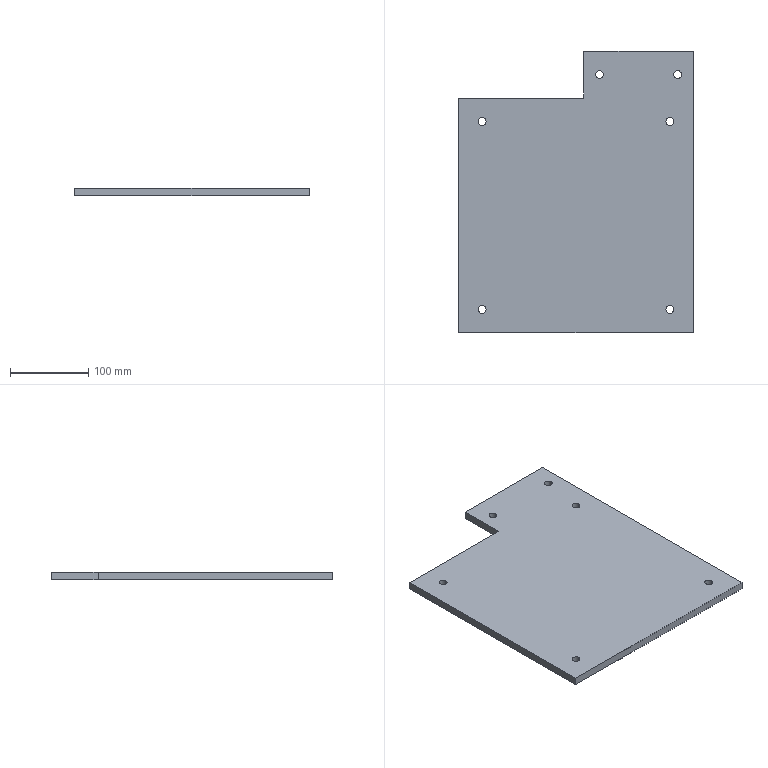Part | SolidWorks | features ICE 2, Extrusion 1 | 1 solid | 20 faces | box 300 x 360 x 10 mm | volume 979288 mm3 | cylinder 12 | plane 8 | commonest cylinder face diameters 10 x12
STEP:
#1=CARTESIAN_POINT('',(275.,330.,0.));
#2=VERTEX_POINT('',#1);
#3=CARTESIAN_POINT('',(285.,330.,0.));
#4=VERTEX_POINT('',#3);
#5=CARTESIAN_POINT('',(280.,330.,0.));
#6=DIRECTION('',(0.,0.,1.));
#7=DIRECTION('',(1.,0.,0.));
#8=AXIS2_PLACEMENT_3D('',#5,#6,#7);
#9=CIRCLE('',#8,5.);
#10=EDGE_CURVE('',#2,#4,#9,.T.);
#11=ORIENTED_EDGE('',*,*,#10,.F.);
#12=CARTESIAN_POINT('',(275.,330.,10.));
#13=VERTEX_POINT('',#12);
#14=CARTESIAN_POINT('',(275.,330.,-30.));
#15=DIRECTION('',(0.,0.,1.));
#16=VECTOR('',#15,1000.);
#17=LINE('',#14,#16);
#18=EDGE_CURVE('',#2,#13,#17,.T.);
#19=ORIENTED_EDGE('',*,*,#18,.T.);
#20=CARTESIAN_POINT('',(285.,330.,10.));
#21=VERTEX_POINT('',#20);
#22=CARTESIAN_POINT('',(280.,330.,10.));
#23=DIRECTION('',(0.,0.,1.));
#24=DIRECTION('',(1.,0.,0.));
#25=AXIS2_PLACEMENT_3D('',#22,#23,#24);
#26=CIRCLE('',#25,5.);
#27=EDGE_CURVE('',#13,#21,#26,.T.);
#28=ORIENTED_EDGE('',*,*,#27,.T.);
#29=CARTESIAN_POINT('',(285.,330.,-30.));
#30=DIRECTION('',(0.,0.,1.));
#31=VECTOR('',#30,1000.);
#32=LINE('',#29,#31);
#33=EDGE_CURVE('',#4,#21,#32,.T.);
#34=ORIENTED_EDGE('',*,*,#33,.F.);
#35=EDGE_LOOP('',(#11,#19,#28,#34));
#36=FACE_OUTER_BOUND('',#35,.T.);
#37=CARTESIAN_POINT('',(280.,330.,-30.));
#38=DIRECTION('',(0.,0.,1.));
#39=DIRECTION('',(1.,0.,0.));
#40=AXIS2_PLACEMENT_3D('',#37,#38,#39);
#41=CYLINDRICAL_SURFACE('',#40,5.);
#42=ADVANCED_FACE('',(#36),#41,.F.);
#43=CARTESIAN_POINT('',(185.,330.,0.));
#44=VERTEX_POINT('',#43);
#45=CARTESIAN_POINT('',(175.,330.,0.));
#46=VERTEX_POINT('',#45);
#47=CARTESIAN_POINT('',(180.,330.,0.));
#48=DIRECTION('',(0.,0.,-1.));
#49=DIRECTION('',(1.,0.,0.));
#50=AXIS2_PLACEMENT_3D('',#47,#48,#49);
#51=CIRCLE('',#50,5.);
#52=EDGE_CURVE('',#44,#46,#51,.T.);
#53=ORIENTED_EDGE('',*,*,#52,.T.);
#54=CARTESIAN_POINT('',(175.,330.,10.));
#55=VERTEX_POINT('',#54);
#56=CARTESIAN_POINT('',(175.,330.,-30.));
#57=DIRECTION('',(0.,0.,1.));
#58=VECTOR('',#57,1000.);
#59=LINE('',#56,#58);
#60=EDGE_CURVE('',#46,#55,#59,.T.);
#61=ORIENTED_EDGE('',*,*,#60,.T.);
#62=CARTESIAN_POINT('',(185.,330.,10.));
#63=VERTEX_POINT('',#62);
#64=CARTESIAN_POINT('',(180.,330.,10.));
#65=DIRECTION('',(0.,0.,-1.));
#66=DIRECTION('',(1.,0.,0.));
#67=AXIS2_PLACEMENT_3D('',#64,#65,#66);
#68=CIRCLE('',#67,5.);
#69=EDGE_CURVE('',#63,#55,#68,.T.);
#70=ORIENTED_EDGE('',*,*,#69,.F.);
#71=CARTESIAN_POINT('',(185.,330.,-30.));
#72=DIRECTION('',(0.,0.,1.));
#73=VECTOR('',#72,1000.);
#74=LINE('',#71,#73);
#75=EDGE_CURVE('',#44,#63,#74,.T.);
#76=ORIENTED_EDGE('',*,*,#75,.F.);
#77=EDGE_LOOP('',(#53,#61,#70,#76));
#78=FACE_OUTER_BOUND('',#77,.T.);
#79=CARTESIAN_POINT('',(180.,330.,-30.));
#80=DIRECTION('',(0.,0.,1.));
#81=DIRECTION('',(1.,0.,0.));
#82=AXIS2_PLACEMENT_3D('',#79,#80,#81);
#83=CYLINDRICAL_SURFACE('',#82,5.);
#84=ADVANCED_FACE('',(#78),#83,.F.);
#85=CARTESIAN_POINT('',(35.,270.,10.));
#86=VERTEX_POINT('',#85);
#87=CARTESIAN_POINT('',(25.,270.,10.));
#88=VERTEX_POINT('',#87);
#89=CARTESIAN_POINT('',(30.,270.,10.));
#90=DIRECTION('',(0.,0.,-1.));
#91=DIRECTION('',(1.,0.,0.));
#92=AXIS2_PLACEMENT_3D('',#89,#90,#91);
#93=CIRCLE('',#92,5.);
#94=EDGE_CURVE('',#86,#88,#93,.T.);
#95=ORIENTED_EDGE('',*,*,#94,.F.);
#96=CARTESIAN_POINT('',(35.,270.,0.));
#97=VERTEX_POINT('',#96);
#98=CARTESIAN_POINT('',(35.,270.,10.));
#99=DIRECTION('',(0.,0.,-1.));
#100=VECTOR('',#99,1000.);
#101=LINE('',#98,#100);
#102=EDGE_CURVE('',#86,#97,#101,.T.);
#103=ORIENTED_EDGE('',*,*,#102,.T.);
#104=CARTESIAN_POINT('',(25.,270.,0.));
#105=VERTEX_POINT('',#104);
#106=CARTESIAN_POINT('',(30.,270.,0.));
#107=DIRECTION('',(0.,0.,-1.));
#108=DIRECTION('',(1.,0.,0.));
#109=AXIS2_PLACEMENT_3D('',#106,#107,#108);
#110=CIRCLE('',#109,5.);
#111=EDGE_CURVE('',#97,#105,#110,.T.);
#112=ORIENTED_EDGE('',*,*,#111,.T.);
#113=CARTESIAN_POINT('',(25.,270.,10.));
#114=DIRECTION('',(0.,0.,-1.));
#115=VECTOR('',#114,1000.);
#116=LINE('',#113,#115);
#117=EDGE_CURVE('',#88,#105,#116,.T.);
#118=ORIENTED_EDGE('',*,*,#117,.F.);
#119=EDGE_LOOP('',(#95,#103,#112,#118));
#120=FACE_OUTER_BOUND('',#119,.T.);
#121=CARTESIAN_POINT('',(30.,270.,10.));
#122=DIRECTION('',(0.,0.,-1.));
#123=DIRECTION('',(-1.,0.,0.));
#124=AXIS2_PLACEMENT_3D('',#121,#122,#123);
#125=CYLINDRICAL_SURFACE('',#124,5.);
#126=ADVANCED_FACE('',(#120),#125,.F.);
#127=CARTESIAN_POINT('',(275.,30.,10.));
#128=VERTEX_POINT('',#127);
#129=CARTESIAN_POINT('',(265.,30.,10.));
#130=VERTEX_POINT('',#129);
#131=CARTESIAN_POINT('',(270.,30.,10.));
#132=DIRECTION('',(0.,0.,-1.));
#133=DIRECTION('',(1.,0.,0.));
#134=AXIS2_PLACEMENT_3D('',#131,#132,#133);
#135=CIRCLE('',#134,5.);
#136=EDGE_CURVE('',#128,#130,#135,.T.);
#137=ORIENTED_EDGE('',*,*,#136,.F.);
#138=CARTESIAN_POINT('',(275.,30.,0.));
#139=VERTEX_POINT('',#138);
#140=CARTESIAN_POINT('',(275.,30.,10.));
#141=DIRECTION('',(0.,0.,-1.));
#142=VECTOR('',#141,1000.);
#143=LINE('',#140,#142);
#144=EDGE_CURVE('',#128,#139,#143,.T.);
#145=ORIENTED_EDGE('',*,*,#144,.T.);
#146=CARTESIAN_POINT('',(265.,30.,0.));
#147=VERTEX_POINT('',#146);
#148=CARTESIAN_POINT('',(270.,30.,0.));
#149=DIRECTION('',(0.,0.,-1.));
#150=DIRECTION('',(1.,0.,0.));
#151=AXIS2_PLACEMENT_3D('',#148,#149,#150);
#152=CIRCLE('',#151,5.);
#153=EDGE_CURVE('',#139,#147,#152,.T.);
#154=ORIENTED_EDGE('',*,*,#153,.T.);
#155=CARTESIAN_POINT('',(265.,30.,10.));
#156=DIRECTION('',(0.,0.,-1.));
#157=VECTOR('',#156,1000.);
#158=LINE('',#155,#157);
#159=EDGE_CURVE('',#130,#147,#158,.T.);
#160=ORIENTED_EDGE('',*,*,#159,.F.);
#161=EDGE_LOOP('',(#137,#145,#154,#160));
#162=FACE_OUTER_BOUND('',#161,.T.);
#163=CARTESIAN_POINT('',(270.,30.,10.));
#164=DIRECTION('',(0.,0.,-1.));
#165=DIRECTION('',(-1.,0.,0.));
#166=AXIS2_PLACEMENT_3D('',#163,#164,#165);
#167=CYLINDRICAL_SURFACE('',#166,5.);
#168=ADVANCED_FACE('',(#162),#167,.F.);
#169=CARTESIAN_POINT('',(25.,30.,10.));
#170=VERTEX_POINT('',#169);
#171=CARTESIAN_POINT('',(35.,30.,10.));
#172=VERTEX_POINT('',#171);
#173=CARTESIAN_POINT('',(30.,30.,10.));
#174=DIRECTION('',(0.,0.,1.));
#175=DIRECTION('',(1.,0.,0.));
#176=AXIS2_PLACEMENT_3D('',#173,#174,#175);
#177=CIRCLE('',#176,5.);
#178=EDGE_CURVE('',#170,#172,#177,.T.);
#179=ORIENTED_EDGE('',*,*,#178,.T.);
#180=CARTESIAN_POINT('',(35.,30.,0.));
#181=VERTEX_POINT('',#180);
#182=CARTESIAN_POINT('',(35.,30.,10.));
#183=DIRECTION('',(0.,0.,-1.));
#184=VECTOR('',#183,1000.);
#185=LINE('',#182,#184);
#186=EDGE_CURVE('',#172,#181,#185,.T.);
#187=ORIENTED_EDGE('',*,*,#186,.T.);
#188=CARTESIAN_POINT('',(25.,30.,0.));
#189=VERTEX_POINT('',#188);
#190=CARTESIAN_POINT('',(30.,30.,0.));
#191=DIRECTION('',(0.,0.,1.));
#192=DIRECTION('',(1.,0.,0.));
#193=AXIS2_PLACEMENT_3D('',#190,#191,#192);
#194=CIRCLE('',#193,5.);
#195=EDGE_CURVE('',#189,#181,#194,.T.);
#196=ORIENTED_EDGE('',*,*,#195,.F.);
#197=CARTESIAN_POINT('',(25.,30.,10.));
#198=DIRECTION('',(0.,0.,-1.));
#199=VECTOR('',#198,1000.);
#200=LINE('',#197,#199);
#201=EDGE_CURVE('',#170,#189,#200,.T.);
#202=ORIENTED_EDGE('',*,*,#201,.F.);
#203=EDGE_LOOP('',(#179,#187,#196,#202));
#204=FACE_OUTER_BOUND('',#203,.T.);
#205=CARTESIAN_POINT('',(30.,30.,10.));
#206=DIRECTION('',(0.,0.,-1.));
#207=DIRECTION('',(-1.,0.,0.));
#208=AXIS2_PLACEMENT_3D('',#205,#206,#207);
#209=CYLINDRICAL_SURFACE('',#208,5.);
#210=ADVANCED_FACE('',(#204),#209,.F.);
#211=CARTESIAN_POINT('',(265.,270.,10.));
#212=VERTEX_POINT('',#211);
#213=CARTESIAN_POINT('',(275.,270.,10.));
#214=VERTEX_POINT('',#213);
#215=CARTESIAN_POINT('',(270.,270.,10.));
#216=DIRECTION('',(0.,0.,1.));
#217=DIRECTION('',(1.,0.,0.));
#218=AXIS2_PLACEMENT_3D('',#215,#216,#217);
#219=CIRCLE('',#218,5.);
#220=EDGE_CURVE('',#212,#214,#219,.T.);
#221=ORIENTED_EDGE('',*,*,#220,.T.);
#222=CARTESIAN_POINT('',(275.,270.,0.));
#223=VERTEX_POINT('',#222);
#224=CARTESIAN_POINT('',(275.,270.,10.));
#225=DIRECTION('',(0.,0.,-1.));
#226=VECTOR('',#225,1000.);
#227=LINE('',#224,#226);
#228=EDGE_CURVE('',#214,#223,#227,.T.);
#229=ORIENTED_EDGE('',*,*,#228,.T.);
#230=CARTESIAN_POINT('',(265.,270.,0.));
#231=VERTEX_POINT('',#230);
#232=CARTESIAN_POINT('',(270.,270.,0.));
#233=DIRECTION('',(0.,0.,1.));
#234=DIRECTION('',(1.,0.,0.));
#235=AXIS2_PLACEMENT_3D('',#232,#233,#234);
#236=CIRCLE('',#235,5.);
#237=EDGE_CURVE('',#231,#223,#236,.T.);
#238=ORIENTED_EDGE('',*,*,#237,.F.);
#239=CARTESIAN_POINT('',(265.,270.,10.));
#240=DIRECTION('',(0.,0.,-1.));
#241=VECTOR('',#240,1000.);
#242=LINE('',#239,#241);
#243=EDGE_CURVE('',#212,#231,#242,.T.);
#244=ORIENTED_EDGE('',*,*,#243,.F.);
#245=EDGE_LOOP('',(#221,#229,#238,#244));
#246=FACE_OUTER_BOUND('',#245,.T.);
#247=CARTESIAN_POINT('',(270.,270.,10.));
#248=DIRECTION('',(0.,0.,-1.));
#249=DIRECTION('',(-1.,0.,0.));
#250=AXIS2_PLACEMENT_3D('',#247,#248,#249);
#251=CYLINDRICAL_SURFACE('',#250,5.);
#252=ADVANCED_FACE('',(#246),#251,.F.);
#253=CARTESIAN_POINT('',(280.,330.,10.));
#254=DIRECTION('',(0.,0.,1.));
#255=DIRECTION('',(1.,0.,0.));
#256=AXIS2_PLACEMENT_3D('',#253,#254,#255);
#257=CIRCLE('',#256,5.);
#258=EDGE_CURVE('',#21,#13,#257,.T.);
#259=ORIENTED_EDGE('',*,*,#258,.F.);
#260=ORIENTED_EDGE('',*,*,#27,.F.);
#261=EDGE_LOOP('',(#259,#260));
#262=FACE_BOUND('',#261,.T.);
#263=CARTESIAN_POINT('',(30.,270.,10.));
#264=DIRECTION('',(0.,0.,-1.));
#265=DIRECTION('',(1.,0.,0.));
#266=AXIS2_PLACEMENT_3D('',#263,#264,#265);
#267=CIRCLE('',#266,5.);
#268=EDGE_CURVE('',#88,#86,#267,.T.);
#269=ORIENTED_EDGE('',*,*,#268,.T.);
#270=ORIENTED_EDGE('',*,*,#94,.T.);
#271=EDGE_LOOP('',(#269,#270));
#272=FACE_BOUND('',#271,.T.);
#273=ORIENTED_EDGE('',*,*,#220,.F.);
#274=CARTESIAN_POINT('',(270.,270.,10.));
#275=DIRECTION('',(0.,0.,1.));
#276=DIRECTION('',(1.,0.,0.));
#277=AXIS2_PLACEMENT_3D('',#274,#275,#276);
#278=CIRCLE('',#277,5.);
#279=EDGE_CURVE('',#214,#212,#278,.T.);
#280=ORIENTED_EDGE('',*,*,#279,.F.);
#281=EDGE_LOOP('',(#273,#280));
#282=FACE_BOUND('',#281,.T.);
#283=ORIENTED_EDGE('',*,*,#178,.F.);
#284=CARTESIAN_POINT('',(30.,30.,10.));
#285=DIRECTION('',(0.,0.,1.));
#286=DIRECTION('',(1.,0.,0.));
#287=AXIS2_PLACEMENT_3D('',#284,#285,#286);
#288=CIRCLE('',#287,5.);
#289=EDGE_CURVE('',#172,#170,#288,.T.);
#290=ORIENTED_EDGE('',*,*,#289,.F.);
#291=EDGE_LOOP('',(#283,#290));
#292=FACE_BOUND('',#291,.T.);
#293=CARTESIAN_POINT('',(270.,30.,10.));
#294=DIRECTION('',(0.,0.,-1.));
#295=DIRECTION('',(1.,0.,0.));
#296=AXIS2_PLACEMENT_3D('',#293,#294,#295);
#297=CIRCLE('',#296,5.);
#298=EDGE_CURVE('',#130,#128,#297,.T.);
#299=ORIENTED_EDGE('',*,*,#298,.T.);
#300=ORIENTED_EDGE('',*,*,#136,.T.);
#301=EDGE_LOOP('',(#299,#300));
#302=FACE_BOUND('',#301,.T.);
#303=CARTESIAN_POINT('',(160.,300.,10.));
#304=VERTEX_POINT('',#303);
#305=CARTESIAN_POINT('',(160.,360.,10.));
#306=VERTEX_POINT('',#305);
#307=CARTESIAN_POINT('',(160.,300.,10.));
#308=DIRECTION('',(0.,1.,0.));
#309=VECTOR('',#308,1000.);
#310=LINE('',#307,#309);
#311=EDGE_CURVE('',#304,#306,#310,.T.);
#312=ORIENTED_EDGE('',*,*,#311,.F.);
#313=CARTESIAN_POINT('',(0.,300.,10.));
#314=VERTEX_POINT('',#313);
#315=CARTESIAN_POINT('',(0.,300.,10.));
#316=DIRECTION('',(-1.,0.,0.));
#317=VECTOR('',#316,1000.);
#318=LINE('',#315,#317);
#319=EDGE_CURVE('',#304,#314,#318,.T.);
#320=ORIENTED_EDGE('',*,*,#319,.T.);
#321=CARTESIAN_POINT('',(0.,0.,10.));
#322=VERTEX_POINT('',#321);
#323=CARTESIAN_POINT('',(0.,0.,10.));
#324=DIRECTION('',(0.,-1.,0.));
#325=VECTOR('',#324,1000.);
#326=LINE('',#323,#325);
#327=EDGE_CURVE('',#314,#322,#326,.T.);
#328=ORIENTED_EDGE('',*,*,#327,.T.);
#329=CARTESIAN_POINT('',(300.,0.,10.));
#330=VERTEX_POINT('',#329);
#331=CARTESIAN_POINT('',(0.,0.,10.));
#332=DIRECTION('',(1.,0.,0.));
#333=VECTOR('',#332,1000.);
#334=LINE('',#331,#333);
#335=EDGE_CURVE('',#322,#330,#334,.T.);
#336=ORIENTED_EDGE('',*,*,#335,.T.);
#337=CARTESIAN_POINT('',(300.,360.,10.));
#338=VERTEX_POINT('',#337);
#339=CARTESIAN_POINT('',(300.,0.,10.));
#340=DIRECTION('',(0.,1.,0.));
#341=VECTOR('',#340,1000.);
#342=LINE('',#339,#341);
#343=EDGE_CURVE('',#330,#338,#342,.T.);
#344=ORIENTED_EDGE('',*,*,#343,.T.);
#345=CARTESIAN_POINT('',(0.,360.,10.));
#346=DIRECTION('',(-1.,0.,0.));
#347=VECTOR('',#346,1000.);
#348=LINE('',#345,#347);
#349=EDGE_CURVE('',#338,#306,#348,.T.);
#350=ORIENTED_EDGE('',*,*,#349,.T.);
#351=EDGE_LOOP('',(#312,#320,#328,#336,#344,#350));
#352=FACE_OUTER_BOUND('',#351,.T.);
#353=ORIENTED_EDGE('',*,*,#69,.T.);
#354=CARTESIAN_POINT('',(180.,330.,10.));
#355=DIRECTION('',(0.,0.,-1.));
#356=DIRECTION('',(1.,0.,0.));
#357=AXIS2_PLACEMENT_3D('',#354,#355,#356);
#358=CIRCLE('',#357,5.);
#359=EDGE_CURVE('',#55,#63,#358,.T.);
#360=ORIENTED_EDGE('',*,*,#359,.T.);
#361=EDGE_LOOP('',(#353,#360));
#362=FACE_BOUND('',#361,.T.);
#363=CARTESIAN_POINT('',(0.,0.,10.));
#364=DIRECTION('',(0.,0.,1.));
#365=DIRECTION('',(1.,0.,0.));
#366=AXIS2_PLACEMENT_3D('',#363,#364,#365);
#367=PLANE('',#366);
#368=ADVANCED_FACE('',(#262,#272,#282,#292,#302,#352,#362),#367,.T.);
#369=CARTESIAN_POINT('',(280.,330.,0.));
#370=DIRECTION('',(0.,0.,1.));
#371=DIRECTION('',(1.,0.,0.));
#372=AXIS2_PLACEMENT_3D('',#369,#370,#371);
#373=CIRCLE('',#372,5.);
#374=EDGE_CURVE('',#4,#2,#373,.T.);
#375=ORIENTED_EDGE('',*,*,#374,.T.);
#376=ORIENTED_EDGE('',*,*,#10,.T.);
#377=EDGE_LOOP('',(#375,#376));
#378=FACE_BOUND('',#377,.T.);
#379=CARTESIAN_POINT('',(30.,270.,0.));
#380=DIRECTION('',(0.,0.,-1.));
#381=DIRECTION('',(1.,0.,0.));
#382=AXIS2_PLACEMENT_3D('',#379,#380,#381);
#383=CIRCLE('',#382,5.);
#384=EDGE_CURVE('',#105,#97,#383,.T.);
#385=ORIENTED_EDGE('',*,*,#384,.F.);
#386=ORIENTED_EDGE('',*,*,#111,.F.);
#387=EDGE_LOOP('',(#385,#386));
#388=FACE_BOUND('',#387,.T.);
#389=ORIENTED_EDGE('',*,*,#237,.T.);
#390=CARTESIAN_POINT('',(270.,270.,0.));
#391=DIRECTION('',(0.,0.,1.));
#392=DIRECTION('',(1.,0.,0.));
#393=AXIS2_PLACEMENT_3D('',#390,#391,#392);
#394=CIRCLE('',#393,5.);
#395=EDGE_CURVE('',#223,#231,#394,.T.);
#396=ORIENTED_EDGE('',*,*,#395,.T.);
#397=EDGE_LOOP('',(#389,#396));
#398=FACE_BOUND('',#397,.T.);
#399=ORIENTED_EDGE('',*,*,#195,.T.);
#400=CARTESIAN_POINT('',(30.,30.,0.));
#401=DIRECTION('',(0.,0.,1.));
#402=DIRECTION('',(1.,0.,0.));
#403=AXIS2_PLACEMENT_3D('',#400,#401,#402);
#404=CIRCLE('',#403,5.);
#405=EDGE_CURVE('',#181,#189,#404,.T.);
#406=ORIENTED_EDGE('',*,*,#405,.T.);
#407=EDGE_LOOP('',(#399,#406));
#408=FACE_BOUND('',#407,.T.);
#409=CARTESIAN_POINT('',(270.,30.,0.));
#410=DIRECTION('',(0.,0.,-1.));
#411=DIRECTION('',(1.,0.,0.));
#412=AXIS2_PLACEMENT_3D('',#409,#410,#411);
#413=CIRCLE('',#412,5.);
#414=EDGE_CURVE('',#147,#139,#413,.T.);
#415=ORIENTED_EDGE('',*,*,#414,.F.);
#416=ORIENTED_EDGE('',*,*,#153,.F.);
#417=EDGE_LOOP('',(#415,#416));
#418=FACE_BOUND('',#417,.T.);
#419=CARTESIAN_POINT('',(160.,300.,0.));
#420=VERTEX_POINT('',#419);
#421=CARTESIAN_POINT('',(0.,300.,0.));
#422=VERTEX_POINT('',#421);
#423=CARTESIAN_POINT('',(0.,300.,0.));
#424=DIRECTION('',(-1.,0.,0.));
#425=VECTOR('',#424,1000.);
#426=LINE('',#423,#425);
#427=EDGE_CURVE('',#420,#422,#426,.T.);
#428=ORIENTED_EDGE('',*,*,#427,.F.);
#429=CARTESIAN_POINT('',(160.,360.,0.));
#430=VERTEX_POINT('',#429);
#431=CARTESIAN_POINT('',(160.,360.,0.));
#432=DIRECTION('',(0.,-1.,0.));
#433=VECTOR('',#432,1000.);
#434=LINE('',#431,#433);
#435=EDGE_CURVE('',#430,#420,#434,.T.);
#436=ORIENTED_EDGE('',*,*,#435,.F.);
#437=CARTESIAN_POINT('',(300.,360.,0.));
#438=VERTEX_POINT('',#437);
#439=CARTESIAN_POINT('',(0.,360.,0.));
#440=DIRECTION('',(-1.,0.,0.));
#441=VECTOR('',#440,1000.);
#442=LINE('',#439,#441);
#443=EDGE_CURVE('',#438,#430,#442,.T.);
#444=ORIENTED_EDGE('',*,*,#443,.F.);
#445=CARTESIAN_POINT('',(300.,0.,0.));
#446=VERTEX_POINT('',#445);
#447=CARTESIAN_POINT('',(300.,0.,0.));
#448=DIRECTION('',(0.,1.,0.));
#449=VECTOR('',#448,1000.);
#450=LINE('',#447,#449);
#451=EDGE_CURVE('',#446,#438,#450,.T.);
#452=ORIENTED_EDGE('',*,*,#451,.F.);
#453=CARTESIAN_POINT('',(0.,0.,0.));
#454=VERTEX_POINT('',#453);
#455=CARTESIAN_POINT('',(0.,0.,0.));
#456=DIRECTION('',(1.,0.,0.));
#457=VECTOR('',#456,1000.);
#458=LINE('',#455,#457);
#459=EDGE_CURVE('',#454,#446,#458,.T.);
#460=ORIENTED_EDGE('',*,*,#459,.F.);
#461=CARTESIAN_POINT('',(0.,0.,0.));
#462=DIRECTION('',(0.,-1.,0.));
#463=VECTOR('',#462,1000.);
#464=LINE('',#461,#463);
#465=EDGE_CURVE('',#422,#454,#464,.T.);
#466=ORIENTED_EDGE('',*,*,#465,.F.);
#467=EDGE_LOOP('',(#428,#436,#444,#452,#460,#466));
#468=FACE_OUTER_BOUND('',#467,.T.);
#469=ORIENTED_EDGE('',*,*,#52,.F.);
#470=CARTESIAN_POINT('',(180.,330.,0.));
#471=DIRECTION('',(0.,0.,-1.));
#472=DIRECTION('',(1.,0.,0.));
#473=AXIS2_PLACEMENT_3D('',#470,#471,#472);
#474=CIRCLE('',#473,5.);
#475=EDGE_CURVE('',#46,#44,#474,.T.);
#476=ORIENTED_EDGE('',*,*,#475,.F.);
#477=EDGE_LOOP('',(#469,#476));
#478=FACE_BOUND('',#477,.T.);
#479=CARTESIAN_POINT('',(0.,0.,0.));
#480=DIRECTION('',(0.,0.,1.));
#481=DIRECTION('',(1.,0.,0.));
#482=AXIS2_PLACEMENT_3D('',#479,#480,#481);
#483=PLANE('',#482);
#484=ADVANCED_FACE('',(#378,#388,#398,#408,#418,#468,#478),#483,.F.);
#485=ORIENTED_EDGE('',*,*,#443,.T.);
#486=CARTESIAN_POINT('',(160.,360.,10.));
#487=DIRECTION('',(0.,0.,-1.));
#488=VECTOR('',#487,1000.);
#489=LINE('',#486,#488);
#490=EDGE_CURVE('',#306,#430,#489,.T.);
#491=ORIENTED_EDGE('',*,*,#490,.F.);
#492=ORIENTED_EDGE('',*,*,#349,.F.);
#493=CARTESIAN_POINT('',(300.,360.,10.));
#494=DIRECTION('',(0.,0.,-1.));
#495=VECTOR('',#494,1000.);
#496=LINE('',#493,#495);
#497=EDGE_CURVE('',#338,#438,#496,.T.);
#498=ORIENTED_EDGE('',*,*,#497,.T.);
#499=EDGE_LOOP('',(#485,#491,#492,#498));
#500=FACE_OUTER_BOUND('',#499,.T.);
#501=CARTESIAN_POINT('',(0.,360.,10.));
#502=DIRECTION('',(0.,-1.,0.));
#503=DIRECTION('',(0.,0.,-1.));
#504=AXIS2_PLACEMENT_3D('',#501,#502,#503);
#505=PLANE('',#504);
#506=ADVANCED_FACE('',(#500),#505,.F.);
#507=ORIENTED_EDGE('',*,*,#319,.F.);
#508=CARTESIAN_POINT('',(160.,300.,0.));
#509=DIRECTION('',(0.,0.,1.));
#510=VECTOR('',#509,1000.);
#511=LINE('',#508,#510);
#512=EDGE_CURVE('',#420,#304,#511,.T.);
#513=ORIENTED_EDGE('',*,*,#512,.F.);
#514=ORIENTED_EDGE('',*,*,#427,.T.);
#515=CARTESIAN_POINT('',(0.,300.,10.));
#516=DIRECTION('',(0.,0.,-1.));
#517=VECTOR('',#516,1000.);
#518=LINE('',#515,#517);
#519=EDGE_CURVE('',#314,#422,#518,.T.);
#520=ORIENTED_EDGE('',*,*,#519,.F.);
#521=EDGE_LOOP('',(#507,#513,#514,#520));
#522=FACE_OUTER_BOUND('',#521,.T.);
#523=CARTESIAN_POINT('',(0.,300.,10.));
#524=DIRECTION('',(0.,-1.,0.));
#525=DIRECTION('',(0.,0.,-1.));
#526=AXIS2_PLACEMENT_3D('',#523,#524,#525);
#527=PLANE('',#526);
#528=ADVANCED_FACE('',(#522),#527,.F.);
#529=ORIENTED_EDGE('',*,*,#465,.T.);
#530=CARTESIAN_POINT('',(0.,0.,10.));
#531=DIRECTION('',(0.,0.,-1.));
#532=VECTOR('',#531,1000.);
#533=LINE('',#530,#532);
#534=EDGE_CURVE('',#322,#454,#533,.T.);
#535=ORIENTED_EDGE('',*,*,#534,.F.);
#536=ORIENTED_EDGE('',*,*,#327,.F.);
#537=ORIENTED_EDGE('',*,*,#519,.T.);
#538=EDGE_LOOP('',(#529,#535,#536,#537));
#539=FACE_OUTER_BOUND('',#538,.T.);
#540=CARTESIAN_POINT('',(0.,0.,10.));
#541=DIRECTION('',(1.,0.,0.));
#542=DIRECTION('',(0.,0.,-1.));
#543=AXIS2_PLACEMENT_3D('',#540,#541,#542);
#544=PLANE('',#543);
#545=ADVANCED_FACE('',(#539),#544,.F.);
#546=ORIENTED_EDGE('',*,*,#459,.T.);
#547=CARTESIAN_POINT('',(300.,0.,10.));
#548=DIRECTION('',(0.,0.,-1.));
#549=VECTOR('',#548,1000.);
#550=LINE('',#547,#549);
#551=EDGE_CURVE('',#330,#446,#550,.T.);
#552=ORIENTED_EDGE('',*,*,#551,.F.);
#553=ORIENTED_EDGE('',*,*,#335,.F.);
#554=ORIENTED_EDGE('',*,*,#534,.T.);
#555=EDGE_LOOP('',(#546,#552,#553,#554));
#556=FACE_OUTER_BOUND('',#555,.T.);
#557=CARTESIAN_POINT('',(0.,0.,10.));
#558=DIRECTION('',(0.,1.,0.));
#559=DIRECTION('',(0.,0.,1.));
#560=AXIS2_PLACEMENT_3D('',#557,#558,#559);
#561=PLANE('',#560);
#562=ADVANCED_FACE('',(#556),#561,.F.);
#563=ORIENTED_EDGE('',*,*,#228,.F.);
#564=ORIENTED_EDGE('',*,*,#279,.T.);
#565=ORIENTED_EDGE('',*,*,#243,.T.);
#566=ORIENTED_EDGE('',*,*,#395,.F.);
#567=EDGE_LOOP('',(#563,#564,#565,#566));
#568=FACE_OUTER_BOUND('',#567,.T.);
#569=CARTESIAN_POINT('',(270.,270.,10.));
#570=DIRECTION('',(0.,0.,-1.));
#571=DIRECTION('',(-1.,0.,0.));
#572=AXIS2_PLACEMENT_3D('',#569,#570,#571);
#573=CYLINDRICAL_SURFACE('',#572,5.);
#574=ADVANCED_FACE('',(#568),#573,.F.);
#575=ORIENTED_EDGE('',*,*,#451,.T.);
#576=ORIENTED_EDGE('',*,*,#497,.F.);
#577=ORIENTED_EDGE('',*,*,#343,.F.);
#578=ORIENTED_EDGE('',*,*,#551,.T.);
#579=EDGE_LOOP('',(#575,#576,#577,#578));
#580=FACE_OUTER_BOUND('',#579,.T.);
#581=CARTESIAN_POINT('',(300.,0.,10.));
#582=DIRECTION('',(-1.,0.,0.));
#583=DIRECTION('',(0.,0.,1.));
#584=AXIS2_PLACEMENT_3D('',#581,#582,#583);
#585=PLANE('',#584);
#586=ADVANCED_FACE('',(#580),#585,.F.);
#587=ORIENTED_EDGE('',*,*,#186,.F.);
#588=ORIENTED_EDGE('',*,*,#289,.T.);
#589=ORIENTED_EDGE('',*,*,#201,.T.);
#590=ORIENTED_EDGE('',*,*,#405,.F.);
#591=EDGE_LOOP('',(#587,#588,#589,#590));
#592=FACE_OUTER_BOUND('',#591,.T.);
#593=CARTESIAN_POINT('',(30.,30.,10.));
#594=DIRECTION('',(0.,0.,-1.));
#595=DIRECTION('',(-1.,0.,0.));
#596=AXIS2_PLACEMENT_3D('',#593,#594,#595);
#597=CYLINDRICAL_SURFACE('',#596,5.);
#598=ADVANCED_FACE('',(#592),#597,.F.);
#599=ORIENTED_EDGE('',*,*,#144,.F.);
#600=ORIENTED_EDGE('',*,*,#298,.F.);
#601=ORIENTED_EDGE('',*,*,#159,.T.);
#602=ORIENTED_EDGE('',*,*,#414,.T.);
#603=EDGE_LOOP('',(#599,#600,#601,#602));
#604=FACE_OUTER_BOUND('',#603,.T.);
#605=CARTESIAN_POINT('',(270.,30.,10.));
#606=DIRECTION('',(0.,0.,-1.));
#607=DIRECTION('',(-1.,0.,0.));
#608=AXIS2_PLACEMENT_3D('',#605,#606,#607);
#609=CYLINDRICAL_SURFACE('',#608,5.);
#610=ADVANCED_FACE('',(#604),#609,.F.);
#611=ORIENTED_EDGE('',*,*,#102,.F.);
#612=ORIENTED_EDGE('',*,*,#268,.F.);
#613=ORIENTED_EDGE('',*,*,#117,.T.);
#614=ORIENTED_EDGE('',*,*,#384,.T.);
#615=EDGE_LOOP('',(#611,#612,#613,#614));
#616=FACE_OUTER_BOUND('',#615,.T.);
#617=CARTESIAN_POINT('',(30.,270.,10.));
#618=DIRECTION('',(0.,0.,-1.));
#619=DIRECTION('',(-1.,0.,0.));
#620=AXIS2_PLACEMENT_3D('',#617,#618,#619);
#621=CYLINDRICAL_SURFACE('',#620,5.);
#622=ADVANCED_FACE('',(#616),#621,.F.);
#623=ORIENTED_EDGE('',*,*,#490,.T.);
#624=ORIENTED_EDGE('',*,*,#435,.T.);
#625=ORIENTED_EDGE('',*,*,#512,.T.);
#626=ORIENTED_EDGE('',*,*,#311,.T.);
#627=EDGE_LOOP('',(#623,#624,#625,#626));
#628=FACE_OUTER_BOUND('',#627,.T.);
#629=CARTESIAN_POINT('',(160.,0.,0.));
#630=DIRECTION('',(-1.,0.,0.));
#631=DIRECTION('',(0.,0.,1.));
#632=AXIS2_PLACEMENT_3D('',#629,#630,#631);
#633=PLANE('',#632);
#634=ADVANCED_FACE('',(#628),#633,.T.);
#635=ORIENTED_EDGE('',*,*,#60,.F.);
#636=ORIENTED_EDGE('',*,*,#475,.T.);
#637=ORIENTED_EDGE('',*,*,#75,.T.);
#638=ORIENTED_EDGE('',*,*,#359,.F.);
#639=EDGE_LOOP('',(#635,#636,#637,#638));
#640=FACE_OUTER_BOUND('',#639,.T.);
#641=CARTESIAN_POINT('',(180.,330.,-30.));
#642=DIRECTION('',(0.,0.,1.));
#643=DIRECTION('',(1.,0.,0.));
#644=AXIS2_PLACEMENT_3D('',#641,#642,#643);
#645=CYLINDRICAL_SURFACE('',#644,5.);
#646=ADVANCED_FACE('',(#640),#645,.F.);
#647=ORIENTED_EDGE('',*,*,#18,.F.);
#648=ORIENTED_EDGE('',*,*,#374,.F.);
#649=ORIENTED_EDGE('',*,*,#33,.T.);
#650=ORIENTED_EDGE('',*,*,#258,.T.);
#651=EDGE_LOOP('',(#647,#648,#649,#650));
#652=FACE_OUTER_BOUND('',#651,.T.);
#653=CARTESIAN_POINT('',(280.,330.,-30.));
#654=DIRECTION('',(0.,0.,1.));
#655=DIRECTION('',(1.,0.,0.));
#656=AXIS2_PLACEMENT_3D('',#653,#654,#655);
#657=CYLINDRICAL_SURFACE('',#656,5.);
#658=ADVANCED_FACE('',(#652),#657,.F.);
#659=CLOSED_SHELL('',(#42,#84,#126,#168,#210,#252,#368,#484,#506,#528,#545,#562,#574,#586,#598,#610,#622,#634,#646,#658));
#660=MANIFOLD_SOLID_BREP('',#659);
#661=CARTESIAN_POINT('',(0.,0.,0.));
#662=DIRECTION('',(0.,0.,1.));
#663=DIRECTION('',(1.,0.,0.));
#664=AXIS2_PLACEMENT_3D('',#661,#662,#663);
#665=(LENGTH_UNIT()NAMED_UNIT(*)SI_UNIT(.MILLI.,.METRE.));
#666=UNCERTAINTY_MEASURE_WITH_UNIT(LENGTH_MEASURE(0.00001),#665,'','');
#667=(NAMED_UNIT(*)PLANE_ANGLE_UNIT()SI_UNIT($,.RADIAN.));
#668=(NAMED_UNIT(*)SI_UNIT($,.STERADIAN.)SOLID_ANGLE_UNIT());
#669=(GEOMETRIC_REPRESENTATION_CONTEXT(3)GLOBAL_UNCERTAINTY_ASSIGNED_CONTEXT((#666))GLOBAL_UNIT_ASSIGNED_CONTEXT((#665,#667,#668))REPRESENTATION_CONTEXT('',''));
#670=ADVANCED_BREP_SHAPE_REPRESENTATION('',(#660,#664),#669);